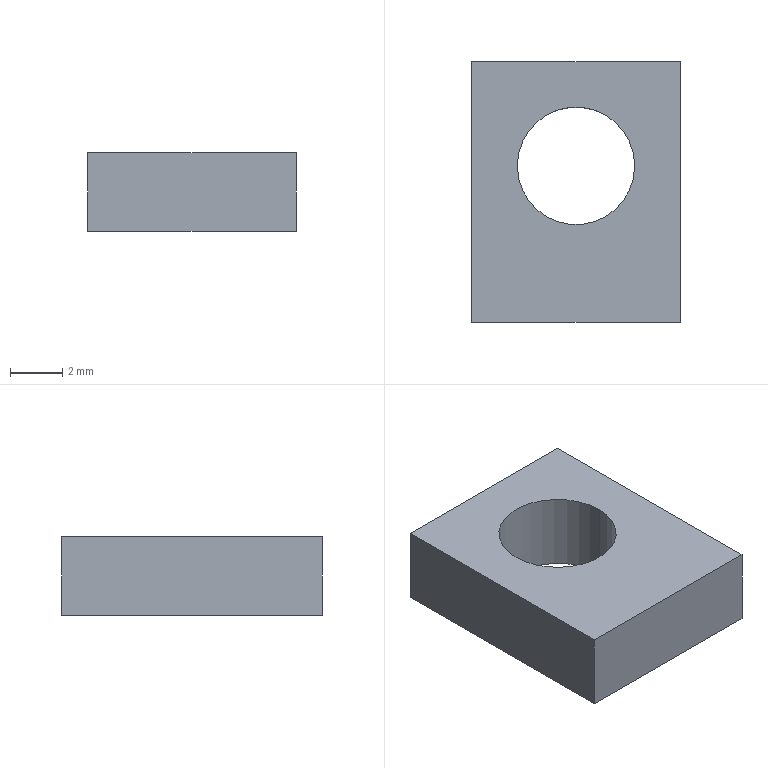Part | STEP file | Stopper plate | 1 solid | 8 faces | box 8 x 10 x 3 mm | volume 192.287 mm3 | plane 6 | cylinder 2 | commonest cylinder face diameters 4.5 x2
STEP:
#1=CARTESIAN_POINT('',(0.,0.,0.));
#2=DIRECTION('',(0.,0.,1.));
#3=DIRECTION('',(1.,0.,0.));
#4=AXIS2_PLACEMENT_3D('',#1,#2,#3);
#5=CARTESIAN_POINT('',(6.25,3.574,0.));
#6=VERTEX_POINT('',#5);
#7=CARTESIAN_POINT('',(6.25,3.574,3.));
#8=VERTEX_POINT('',#7);
#9=CARTESIAN_POINT('',(6.25,3.574,0.));
#10=DIRECTION('',(0.,0.,1.));
#11=VECTOR('',#10,1.);
#12=LINE('',#9,#11);
#13=CARTESIAN_POINT('',(4.,3.574,0.));
#14=DIRECTION('',(0.,0.,1.));
#15=DIRECTION('',(1.,0.,0.));
#16=AXIS2_PLACEMENT_3D('',#13,#14,#15);
#17=CYLINDRICAL_SURFACE('',#16,2.25);
#18=CARTESIAN_POINT('',(6.283,0.));
#19=DIRECTION('',(0.,1.));
#20=VECTOR('',#19,1.);
#21=LINE('',#18,#20);
#22=(GEOMETRIC_REPRESENTATION_CONTEXT(2)PARAMETRIC_REPRESENTATION_CONTEXT()REPRESENTATION_CONTEXT('',''));
#23=DEFINITIONAL_REPRESENTATION('',(#21),#22);
#24=PCURVE('',#17,#23);
#25=CARTESIAN_POINT('',(4.,3.574,0.));
#26=DIRECTION('',(0.,0.,1.));
#27=DIRECTION('',(1.,0.,0.));
#28=AXIS2_PLACEMENT_3D('',#25,#26,#27);
#29=CYLINDRICAL_SURFACE('',#28,2.25);
#30=CARTESIAN_POINT('',(0.,0.));
#31=DIRECTION('',(0.,1.));
#32=VECTOR('',#31,1.);
#33=LINE('',#30,#32);
#34=(GEOMETRIC_REPRESENTATION_CONTEXT(2)PARAMETRIC_REPRESENTATION_CONTEXT()REPRESENTATION_CONTEXT('',''));
#35=DEFINITIONAL_REPRESENTATION('',(#33),#34);
#36=PCURVE('',#29,#35);
#37=SURFACE_CURVE('',#12,(#24,#36),.PCURVE_S1.);
#38=EDGE_CURVE('',#6,#8,#37,.T.);
#39=ORIENTED_EDGE('',*,*,#38,.T.);
#40=CARTESIAN_POINT('',(1.75,3.574,3.));
#41=VERTEX_POINT('',#40);
#42=CARTESIAN_POINT('',(4.,3.574,3.));
#43=DIRECTION('',(0.,0.,1.));
#44=DIRECTION('',(1.,0.,0.));
#45=AXIS2_PLACEMENT_3D('',#42,#43,#44);
#46=CIRCLE('',#45,2.25);
#47=CARTESIAN_POINT('',(0.,3.));
#48=DIRECTION('',(1.,0.));
#49=VECTOR('',#48,1.);
#50=LINE('',#47,#49);
#51=(GEOMETRIC_REPRESENTATION_CONTEXT(2)PARAMETRIC_REPRESENTATION_CONTEXT()REPRESENTATION_CONTEXT('',''));
#52=DEFINITIONAL_REPRESENTATION('',(#50),#51);
#53=PCURVE('',#17,#52);
#54=CARTESIAN_POINT('',(0.,7.574,3.));
#55=DIRECTION('',(0.,0.,-1.));
#56=DIRECTION('',(-1.,0.,0.));
#57=AXIS2_PLACEMENT_3D('',#54,#55,#56);
#58=PLANE('',#57);
#59=CARTESIAN_POINT('',(-6.25,-4.));
#60=CARTESIAN_POINT('',(-6.25,-0.1029));
#61=CARTESIAN_POINT('',(-2.875,-2.051));
#62=CARTESIAN_POINT('',(0.5,-4.));
#63=CARTESIAN_POINT('',(-2.875,-5.949));
#64=CARTESIAN_POINT('',(-6.25,-7.897));
#65=CARTESIAN_POINT('',(-6.25,-4.));
#66=(BOUNDED_CURVE()B_SPLINE_CURVE(2,(#59,#60,#61,#62,#63,#64,#65),.UNSPECIFIED.,.T.,.F.)B_SPLINE_CURVE_WITH_KNOTS((1,2,2,2,2,1),(-2.094,0.,2.094,4.189,6.283,8.378),.UNSPECIFIED.)CURVE()GEOMETRIC_REPRESENTATION_ITEM()RATIONAL_B_SPLINE_CURVE((1.,0.5,1.,0.5,1.,0.5,1.))REPRESENTATION_ITEM(''));
#67=(GEOMETRIC_REPRESENTATION_CONTEXT(2)PARAMETRIC_REPRESENTATION_CONTEXT()REPRESENTATION_CONTEXT('',''));
#68=DEFINITIONAL_REPRESENTATION('',(#66),#67);
#69=PCURVE('',#58,#68);
#70=SURFACE_CURVE('',#46,(#53,#69),.PCURVE_S1.);
#71=EDGE_CURVE('',#41,#8,#70,.T.);
#72=ORIENTED_EDGE('',*,*,#71,.F.);
#73=CARTESIAN_POINT('',(1.75,3.574,0.));
#74=VERTEX_POINT('',#73);
#75=CARTESIAN_POINT('',(1.75,3.574,0.));
#76=DIRECTION('',(0.,0.,1.));
#77=VECTOR('',#76,1.);
#78=LINE('',#75,#77);
#79=CARTESIAN_POINT('',(3.142,0.));
#80=DIRECTION('',(0.,1.));
#81=VECTOR('',#80,1.);
#82=LINE('',#79,#81);
#83=(GEOMETRIC_REPRESENTATION_CONTEXT(2)PARAMETRIC_REPRESENTATION_CONTEXT()REPRESENTATION_CONTEXT('',''));
#84=DEFINITIONAL_REPRESENTATION('',(#82),#83);
#85=PCURVE('',#17,#84);
#86=CARTESIAN_POINT('',(3.142,0.));
#87=DIRECTION('',(0.,1.));
#88=VECTOR('',#87,1.);
#89=LINE('',#86,#88);
#90=(GEOMETRIC_REPRESENTATION_CONTEXT(2)PARAMETRIC_REPRESENTATION_CONTEXT()REPRESENTATION_CONTEXT('',''));
#91=DEFINITIONAL_REPRESENTATION('',(#89),#90);
#92=PCURVE('',#29,#91);
#93=SURFACE_CURVE('',#78,(#85,#92),.PCURVE_S1.);
#94=EDGE_CURVE('',#74,#41,#93,.T.);
#95=ORIENTED_EDGE('',*,*,#94,.F.);
#96=CARTESIAN_POINT('',(4.,3.574,0.));
#97=DIRECTION('',(0.,0.,1.));
#98=DIRECTION('',(1.,0.,0.));
#99=AXIS2_PLACEMENT_3D('',#96,#97,#98);
#100=CIRCLE('',#99,2.25);
#101=CARTESIAN_POINT('',(0.,0.));
#102=DIRECTION('',(1.,0.));
#103=VECTOR('',#102,1.);
#104=LINE('',#101,#103);
#105=(GEOMETRIC_REPRESENTATION_CONTEXT(2)PARAMETRIC_REPRESENTATION_CONTEXT()REPRESENTATION_CONTEXT('',''));
#106=DEFINITIONAL_REPRESENTATION('',(#104),#105);
#107=PCURVE('',#17,#106);
#108=CARTESIAN_POINT('',(0.,7.574,0.));
#109=DIRECTION('',(0.,0.,-1.));
#110=DIRECTION('',(-1.,0.,0.));
#111=AXIS2_PLACEMENT_3D('',#108,#109,#110);
#112=PLANE('',#111);
#113=CARTESIAN_POINT('',(-6.25,-4.));
#114=CARTESIAN_POINT('',(-6.25,-0.1029));
#115=CARTESIAN_POINT('',(-2.875,-2.051));
#116=CARTESIAN_POINT('',(0.5,-4.));
#117=CARTESIAN_POINT('',(-2.875,-5.949));
#118=CARTESIAN_POINT('',(-6.25,-7.897));
#119=CARTESIAN_POINT('',(-6.25,-4.));
#120=(BOUNDED_CURVE()B_SPLINE_CURVE(2,(#113,#114,#115,#116,#117,#118,#119),.UNSPECIFIED.,.T.,.F.)B_SPLINE_CURVE_WITH_KNOTS((1,2,2,2,2,1),(-2.094,0.,2.094,4.189,6.283,8.378),.UNSPECIFIED.)CURVE()GEOMETRIC_REPRESENTATION_ITEM()RATIONAL_B_SPLINE_CURVE((1.,0.5,1.,0.5,1.,0.5,1.))REPRESENTATION_ITEM(''));
#121=(GEOMETRIC_REPRESENTATION_CONTEXT(2)PARAMETRIC_REPRESENTATION_CONTEXT()REPRESENTATION_CONTEXT('',''));
#122=DEFINITIONAL_REPRESENTATION('',(#120),#121);
#123=PCURVE('',#112,#122);
#124=SURFACE_CURVE('',#100,(#107,#123),.PCURVE_S1.);
#125=EDGE_CURVE('',#74,#6,#124,.T.);
#126=ORIENTED_EDGE('',*,*,#125,.T.);
#127=EDGE_LOOP('',(#39,#72,#95,#126));
#128=FACE_BOUND('',#127,.F.);
#129=ADVANCED_FACE('',(#128),#17,.F.);
#130=CARTESIAN_POINT('',(0.,7.574,0.));
#131=VERTEX_POINT('',#130);
#132=CARTESIAN_POINT('',(0.,-2.426,0.));
#133=VERTEX_POINT('',#132);
#134=CARTESIAN_POINT('',(0.,-2.426,0.));
#135=DIRECTION('',(0.,-1.,0.));
#136=VECTOR('',#135,1.);
#137=LINE('',#134,#136);
#138=CARTESIAN_POINT('',(0.,-2.426,3.));
#139=DIRECTION('',(1.,0.,0.));
#140=DIRECTION('',(0.,0.,-1.));
#141=AXIS2_PLACEMENT_3D('',#138,#139,#140);
#142=PLANE('',#141);
#143=CARTESIAN_POINT('',(3.,0.));
#144=DIRECTION('',(0.,-1.));
#145=VECTOR('',#144,1.);
#146=LINE('',#143,#145);
#147=(GEOMETRIC_REPRESENTATION_CONTEXT(2)PARAMETRIC_REPRESENTATION_CONTEXT()REPRESENTATION_CONTEXT('',''));
#148=DEFINITIONAL_REPRESENTATION('',(#146),#147);
#149=PCURVE('',#142,#148);
#150=CARTESIAN_POINT('',(0.,-10.));
#151=DIRECTION('',(0.,-1.));
#152=VECTOR('',#151,1.);
#153=LINE('',#150,#152);
#154=(GEOMETRIC_REPRESENTATION_CONTEXT(2)PARAMETRIC_REPRESENTATION_CONTEXT()REPRESENTATION_CONTEXT('',''));
#155=DEFINITIONAL_REPRESENTATION('',(#153),#154);
#156=PCURVE('',#112,#155);
#157=SURFACE_CURVE('',#137,(#149,#156),.PCURVE_S1.);
#158=EDGE_CURVE('',#131,#133,#157,.T.);
#159=ORIENTED_EDGE('',*,*,#158,.T.);
#160=CARTESIAN_POINT('',(0.,-2.426,3.));
#161=VERTEX_POINT('',#160);
#162=CARTESIAN_POINT('',(0.,-2.426,3.));
#163=DIRECTION('',(0.,0.,-1.));
#164=VECTOR('',#163,1.);
#165=LINE('',#162,#164);
#166=CARTESIAN_POINT('',(0.,0.));
#167=DIRECTION('',(1.,0.));
#168=VECTOR('',#167,1.);
#169=LINE('',#166,#168);
#170=(GEOMETRIC_REPRESENTATION_CONTEXT(2)PARAMETRIC_REPRESENTATION_CONTEXT()REPRESENTATION_CONTEXT('',''));
#171=DEFINITIONAL_REPRESENTATION('',(#169),#170);
#172=PCURVE('',#142,#171);
#173=CARTESIAN_POINT('',(0.,-2.426,3.));
#174=DIRECTION('',(0.,1.,0.));
#175=DIRECTION('',(0.,0.,1.));
#176=AXIS2_PLACEMENT_3D('',#173,#174,#175);
#177=PLANE('',#176);
#178=CARTESIAN_POINT('',(0.,0.));
#179=DIRECTION('',(-1.,0.));
#180=VECTOR('',#179,1.);
#181=LINE('',#178,#180);
#182=(GEOMETRIC_REPRESENTATION_CONTEXT(2)PARAMETRIC_REPRESENTATION_CONTEXT()REPRESENTATION_CONTEXT('',''));
#183=DEFINITIONAL_REPRESENTATION('',(#181),#182);
#184=PCURVE('',#177,#183);
#185=SURFACE_CURVE('',#165,(#172,#184),.PCURVE_S1.);
#186=EDGE_CURVE('',#161,#133,#185,.T.);
#187=ORIENTED_EDGE('',*,*,#186,.F.);
#188=CARTESIAN_POINT('',(0.,7.574,3.));
#189=VERTEX_POINT('',#188);
#190=CARTESIAN_POINT('',(0.,-2.426,3.));
#191=DIRECTION('',(0.,-1.,0.));
#192=VECTOR('',#191,1.);
#193=LINE('',#190,#192);
#194=CARTESIAN_POINT('',(0.,0.));
#195=DIRECTION('',(0.,-1.));
#196=VECTOR('',#195,1.);
#197=LINE('',#194,#196);
#198=(GEOMETRIC_REPRESENTATION_CONTEXT(2)PARAMETRIC_REPRESENTATION_CONTEXT()REPRESENTATION_CONTEXT('',''));
#199=DEFINITIONAL_REPRESENTATION('',(#197),#198);
#200=PCURVE('',#142,#199);
#201=CARTESIAN_POINT('',(0.,-10.));
#202=DIRECTION('',(0.,-1.));
#203=VECTOR('',#202,1.);
#204=LINE('',#201,#203);
#205=(GEOMETRIC_REPRESENTATION_CONTEXT(2)PARAMETRIC_REPRESENTATION_CONTEXT()REPRESENTATION_CONTEXT('',''));
#206=DEFINITIONAL_REPRESENTATION('',(#204),#205);
#207=PCURVE('',#58,#206);
#208=SURFACE_CURVE('',#193,(#200,#207),.PCURVE_S1.);
#209=EDGE_CURVE('',#189,#161,#208,.T.);
#210=ORIENTED_EDGE('',*,*,#209,.F.);
#211=CARTESIAN_POINT('',(0.,7.574,3.));
#212=DIRECTION('',(0.,0.,-1.));
#213=VECTOR('',#212,1.);
#214=LINE('',#211,#213);
#215=CARTESIAN_POINT('',(0.,10.));
#216=DIRECTION('',(1.,0.));
#217=VECTOR('',#216,1.);
#218=LINE('',#215,#217);
#219=(GEOMETRIC_REPRESENTATION_CONTEXT(2)PARAMETRIC_REPRESENTATION_CONTEXT()REPRESENTATION_CONTEXT('',''));
#220=DEFINITIONAL_REPRESENTATION('',(#218),#219);
#221=PCURVE('',#142,#220);
#222=CARTESIAN_POINT('',(0.,7.574,3.));
#223=DIRECTION('',(0.,-1.,0.));
#224=DIRECTION('',(0.,0.,-1.));
#225=AXIS2_PLACEMENT_3D('',#222,#223,#224);
#226=PLANE('',#225);
#227=CARTESIAN_POINT('',(0.,0.));
#228=DIRECTION('',(1.,0.));
#229=VECTOR('',#228,1.);
#230=LINE('',#227,#229);
#231=(GEOMETRIC_REPRESENTATION_CONTEXT(2)PARAMETRIC_REPRESENTATION_CONTEXT()REPRESENTATION_CONTEXT('',''));
#232=DEFINITIONAL_REPRESENTATION('',(#230),#231);
#233=PCURVE('',#226,#232);
#234=SURFACE_CURVE('',#214,(#221,#233),.PCURVE_S1.);
#235=EDGE_CURVE('',#189,#131,#234,.T.);
#236=ORIENTED_EDGE('',*,*,#235,.T.);
#237=EDGE_LOOP('',(#159,#187,#210,#236));
#238=FACE_BOUND('',#237,.T.);
#239=ADVANCED_FACE('',(#238),#142,.F.);
#240=CARTESIAN_POINT('',(8.,-2.426,0.));
#241=VERTEX_POINT('',#240);
#242=CARTESIAN_POINT('',(0.,-2.426,0.));
#243=DIRECTION('',(1.,0.,0.));
#244=VECTOR('',#243,1.);
#245=LINE('',#242,#244);
#246=CARTESIAN_POINT('',(-3.,0.));
#247=DIRECTION('',(0.,1.));
#248=VECTOR('',#247,1.);
#249=LINE('',#246,#248);
#250=(GEOMETRIC_REPRESENTATION_CONTEXT(2)PARAMETRIC_REPRESENTATION_CONTEXT()REPRESENTATION_CONTEXT('',''));
#251=DEFINITIONAL_REPRESENTATION('',(#249),#250);
#252=PCURVE('',#177,#251);
#253=CARTESIAN_POINT('',(0.,-10.));
#254=DIRECTION('',(-1.,0.));
#255=VECTOR('',#254,1.);
#256=LINE('',#253,#255);
#257=(GEOMETRIC_REPRESENTATION_CONTEXT(2)PARAMETRIC_REPRESENTATION_CONTEXT()REPRESENTATION_CONTEXT('',''));
#258=DEFINITIONAL_REPRESENTATION('',(#256),#257);
#259=PCURVE('',#112,#258);
#260=SURFACE_CURVE('',#245,(#252,#259),.PCURVE_S1.);
#261=EDGE_CURVE('',#133,#241,#260,.T.);
#262=ORIENTED_EDGE('',*,*,#261,.T.);
#263=CARTESIAN_POINT('',(8.,-2.426,3.));
#264=VERTEX_POINT('',#263);
#265=CARTESIAN_POINT('',(8.,-2.426,3.));
#266=DIRECTION('',(0.,0.,-1.));
#267=VECTOR('',#266,1.);
#268=LINE('',#265,#267);
#269=CARTESIAN_POINT('',(0.,8.));
#270=DIRECTION('',(-1.,0.));
#271=VECTOR('',#270,1.);
#272=LINE('',#269,#271);
#273=(GEOMETRIC_REPRESENTATION_CONTEXT(2)PARAMETRIC_REPRESENTATION_CONTEXT()REPRESENTATION_CONTEXT('',''));
#274=DEFINITIONAL_REPRESENTATION('',(#272),#273);
#275=PCURVE('',#177,#274);
#276=CARTESIAN_POINT('',(8.,-2.426,3.));
#277=DIRECTION('',(-1.,0.,0.));
#278=DIRECTION('',(0.,0.,1.));
#279=AXIS2_PLACEMENT_3D('',#276,#277,#278);
#280=PLANE('',#279);
#281=CARTESIAN_POINT('',(0.,0.));
#282=DIRECTION('',(-1.,0.));
#283=VECTOR('',#282,1.);
#284=LINE('',#281,#283);
#285=(GEOMETRIC_REPRESENTATION_CONTEXT(2)PARAMETRIC_REPRESENTATION_CONTEXT()REPRESENTATION_CONTEXT('',''));
#286=DEFINITIONAL_REPRESENTATION('',(#284),#285);
#287=PCURVE('',#280,#286);
#288=SURFACE_CURVE('',#268,(#275,#287),.PCURVE_S1.);
#289=EDGE_CURVE('',#264,#241,#288,.T.);
#290=ORIENTED_EDGE('',*,*,#289,.F.);
#291=CARTESIAN_POINT('',(0.,-2.426,3.));
#292=DIRECTION('',(1.,0.,0.));
#293=VECTOR('',#292,1.);
#294=LINE('',#291,#293);
#295=CARTESIAN_POINT('',(0.,0.));
#296=DIRECTION('',(0.,1.));
#297=VECTOR('',#296,1.);
#298=LINE('',#295,#297);
#299=(GEOMETRIC_REPRESENTATION_CONTEXT(2)PARAMETRIC_REPRESENTATION_CONTEXT()REPRESENTATION_CONTEXT('',''));
#300=DEFINITIONAL_REPRESENTATION('',(#298),#299);
#301=PCURVE('',#177,#300);
#302=CARTESIAN_POINT('',(0.,-10.));
#303=DIRECTION('',(-1.,0.));
#304=VECTOR('',#303,1.);
#305=LINE('',#302,#304);
#306=(GEOMETRIC_REPRESENTATION_CONTEXT(2)PARAMETRIC_REPRESENTATION_CONTEXT()REPRESENTATION_CONTEXT('',''));
#307=DEFINITIONAL_REPRESENTATION('',(#305),#306);
#308=PCURVE('',#58,#307);
#309=SURFACE_CURVE('',#294,(#301,#308),.PCURVE_S1.);
#310=EDGE_CURVE('',#161,#264,#309,.T.);
#311=ORIENTED_EDGE('',*,*,#310,.F.);
#312=ORIENTED_EDGE('',*,*,#186,.T.);
#313=EDGE_LOOP('',(#262,#290,#311,#312));
#314=FACE_BOUND('',#313,.T.);
#315=ADVANCED_FACE('',(#314),#177,.F.);
#316=CARTESIAN_POINT('',(8.,7.574,0.));
#317=VERTEX_POINT('',#316);
#318=CARTESIAN_POINT('',(8.,-2.426,0.));
#319=DIRECTION('',(0.,1.,0.));
#320=VECTOR('',#319,1.);
#321=LINE('',#318,#320);
#322=CARTESIAN_POINT('',(-3.,0.));
#323=DIRECTION('',(0.,1.));
#324=VECTOR('',#323,1.);
#325=LINE('',#322,#324);
#326=(GEOMETRIC_REPRESENTATION_CONTEXT(2)PARAMETRIC_REPRESENTATION_CONTEXT()REPRESENTATION_CONTEXT('',''));
#327=DEFINITIONAL_REPRESENTATION('',(#325),#326);
#328=PCURVE('',#280,#327);
#329=CARTESIAN_POINT('',(-8.,-10.));
#330=DIRECTION('',(0.,1.));
#331=VECTOR('',#330,1.);
#332=LINE('',#329,#331);
#333=(GEOMETRIC_REPRESENTATION_CONTEXT(2)PARAMETRIC_REPRESENTATION_CONTEXT()REPRESENTATION_CONTEXT('',''));
#334=DEFINITIONAL_REPRESENTATION('',(#332),#333);
#335=PCURVE('',#112,#334);
#336=SURFACE_CURVE('',#321,(#328,#335),.PCURVE_S1.);
#337=EDGE_CURVE('',#241,#317,#336,.T.);
#338=ORIENTED_EDGE('',*,*,#337,.T.);
#339=CARTESIAN_POINT('',(8.,7.574,3.));
#340=VERTEX_POINT('',#339);
#341=CARTESIAN_POINT('',(8.,7.574,3.));
#342=DIRECTION('',(0.,0.,-1.));
#343=VECTOR('',#342,1.);
#344=LINE('',#341,#343);
#345=CARTESIAN_POINT('',(0.,10.));
#346=DIRECTION('',(-1.,0.));
#347=VECTOR('',#346,1.);
#348=LINE('',#345,#347);
#349=(GEOMETRIC_REPRESENTATION_CONTEXT(2)PARAMETRIC_REPRESENTATION_CONTEXT()REPRESENTATION_CONTEXT('',''));
#350=DEFINITIONAL_REPRESENTATION('',(#348),#349);
#351=PCURVE('',#280,#350);
#352=CARTESIAN_POINT('',(0.,8.));
#353=DIRECTION('',(1.,0.));
#354=VECTOR('',#353,1.);
#355=LINE('',#352,#354);
#356=(GEOMETRIC_REPRESENTATION_CONTEXT(2)PARAMETRIC_REPRESENTATION_CONTEXT()REPRESENTATION_CONTEXT('',''));
#357=DEFINITIONAL_REPRESENTATION('',(#355),#356);
#358=PCURVE('',#226,#357);
#359=SURFACE_CURVE('',#344,(#351,#358),.PCURVE_S1.);
#360=EDGE_CURVE('',#340,#317,#359,.T.);
#361=ORIENTED_EDGE('',*,*,#360,.F.);
#362=CARTESIAN_POINT('',(8.,-2.426,3.));
#363=DIRECTION('',(0.,1.,0.));
#364=VECTOR('',#363,1.);
#365=LINE('',#362,#364);
#366=CARTESIAN_POINT('',(0.,0.));
#367=DIRECTION('',(0.,1.));
#368=VECTOR('',#367,1.);
#369=LINE('',#366,#368);
#370=(GEOMETRIC_REPRESENTATION_CONTEXT(2)PARAMETRIC_REPRESENTATION_CONTEXT()REPRESENTATION_CONTEXT('',''));
#371=DEFINITIONAL_REPRESENTATION('',(#369),#370);
#372=PCURVE('',#280,#371);
#373=CARTESIAN_POINT('',(-8.,-10.));
#374=DIRECTION('',(0.,1.));
#375=VECTOR('',#374,1.);
#376=LINE('',#373,#375);
#377=(GEOMETRIC_REPRESENTATION_CONTEXT(2)PARAMETRIC_REPRESENTATION_CONTEXT()REPRESENTATION_CONTEXT('',''));
#378=DEFINITIONAL_REPRESENTATION('',(#376),#377);
#379=PCURVE('',#58,#378);
#380=SURFACE_CURVE('',#365,(#372,#379),.PCURVE_S1.);
#381=EDGE_CURVE('',#264,#340,#380,.T.);
#382=ORIENTED_EDGE('',*,*,#381,.F.);
#383=ORIENTED_EDGE('',*,*,#289,.T.);
#384=EDGE_LOOP('',(#338,#361,#382,#383));
#385=FACE_BOUND('',#384,.T.);
#386=ADVANCED_FACE('',(#385),#280,.F.);
#387=CARTESIAN_POINT('',(0.,7.574,0.));
#388=DIRECTION('',(-1.,0.,0.));
#389=VECTOR('',#388,1.);
#390=LINE('',#387,#389);
#391=CARTESIAN_POINT('',(3.,0.));
#392=DIRECTION('',(0.,-1.));
#393=VECTOR('',#392,1.);
#394=LINE('',#391,#393);
#395=(GEOMETRIC_REPRESENTATION_CONTEXT(2)PARAMETRIC_REPRESENTATION_CONTEXT()REPRESENTATION_CONTEXT('',''));
#396=DEFINITIONAL_REPRESENTATION('',(#394),#395);
#397=PCURVE('',#226,#396);
#398=CARTESIAN_POINT('',(0.,0.));
#399=DIRECTION('',(1.,0.));
#400=VECTOR('',#399,1.);
#401=LINE('',#398,#400);
#402=(GEOMETRIC_REPRESENTATION_CONTEXT(2)PARAMETRIC_REPRESENTATION_CONTEXT()REPRESENTATION_CONTEXT('',''));
#403=DEFINITIONAL_REPRESENTATION('',(#401),#402);
#404=PCURVE('',#112,#403);
#405=SURFACE_CURVE('',#390,(#397,#404),.PCURVE_S1.);
#406=EDGE_CURVE('',#317,#131,#405,.T.);
#407=ORIENTED_EDGE('',*,*,#406,.T.);
#408=ORIENTED_EDGE('',*,*,#235,.F.);
#409=CARTESIAN_POINT('',(0.,7.574,3.));
#410=DIRECTION('',(-1.,0.,0.));
#411=VECTOR('',#410,1.);
#412=LINE('',#409,#411);
#413=CARTESIAN_POINT('',(0.,0.));
#414=DIRECTION('',(0.,-1.));
#415=VECTOR('',#414,1.);
#416=LINE('',#413,#415);
#417=(GEOMETRIC_REPRESENTATION_CONTEXT(2)PARAMETRIC_REPRESENTATION_CONTEXT()REPRESENTATION_CONTEXT('',''));
#418=DEFINITIONAL_REPRESENTATION('',(#416),#417);
#419=PCURVE('',#226,#418);
#420=CARTESIAN_POINT('',(0.,0.));
#421=DIRECTION('',(1.,0.));
#422=VECTOR('',#421,1.);
#423=LINE('',#420,#422);
#424=(GEOMETRIC_REPRESENTATION_CONTEXT(2)PARAMETRIC_REPRESENTATION_CONTEXT()REPRESENTATION_CONTEXT('',''));
#425=DEFINITIONAL_REPRESENTATION('',(#423),#424);
#426=PCURVE('',#58,#425);
#427=SURFACE_CURVE('',#412,(#419,#426),.PCURVE_S1.);
#428=EDGE_CURVE('',#340,#189,#427,.T.);
#429=ORIENTED_EDGE('',*,*,#428,.F.);
#430=ORIENTED_EDGE('',*,*,#360,.T.);
#431=EDGE_LOOP('',(#407,#408,#429,#430));
#432=FACE_BOUND('',#431,.T.);
#433=ADVANCED_FACE('',(#432),#226,.F.);
#434=CARTESIAN_POINT('',(4.,3.574,3.));
#435=DIRECTION('',(0.,0.,1.));
#436=DIRECTION('',(1.,0.,0.));
#437=AXIS2_PLACEMENT_3D('',#434,#435,#436);
#438=CIRCLE('',#437,2.25);
#439=CARTESIAN_POINT('',(-6.25,-4.));
#440=CARTESIAN_POINT('',(-6.25,-0.1029));
#441=CARTESIAN_POINT('',(-2.875,-2.051));
#442=CARTESIAN_POINT('',(0.5,-4.));
#443=CARTESIAN_POINT('',(-2.875,-5.949));
#444=CARTESIAN_POINT('',(-6.25,-7.897));
#445=CARTESIAN_POINT('',(-6.25,-4.));
#446=(BOUNDED_CURVE()B_SPLINE_CURVE(2,(#439,#440,#441,#442,#443,#444,#445),.UNSPECIFIED.,.T.,.F.)B_SPLINE_CURVE_WITH_KNOTS((1,2,2,2,2,1),(-2.094,0.,2.094,4.189,6.283,8.378),.UNSPECIFIED.)CURVE()GEOMETRIC_REPRESENTATION_ITEM()RATIONAL_B_SPLINE_CURVE((1.,0.5,1.,0.5,1.,0.5,1.))REPRESENTATION_ITEM(''));
#447=(GEOMETRIC_REPRESENTATION_CONTEXT(2)PARAMETRIC_REPRESENTATION_CONTEXT()REPRESENTATION_CONTEXT('',''));
#448=DEFINITIONAL_REPRESENTATION('',(#446),#447);
#449=PCURVE('',#58,#448);
#450=CARTESIAN_POINT('',(0.,3.));
#451=DIRECTION('',(1.,0.));
#452=VECTOR('',#451,1.);
#453=LINE('',#450,#452);
#454=(GEOMETRIC_REPRESENTATION_CONTEXT(2)PARAMETRIC_REPRESENTATION_CONTEXT()REPRESENTATION_CONTEXT('',''));
#455=DEFINITIONAL_REPRESENTATION('',(#453),#454);
#456=PCURVE('',#29,#455);
#457=SURFACE_CURVE('',#438,(#449,#456),.PCURVE_S1.);
#458=EDGE_CURVE('',#8,#41,#457,.T.);
#459=ORIENTED_EDGE('',*,*,#458,.F.);
#460=ORIENTED_EDGE('',*,*,#71,.F.);
#461=EDGE_LOOP('',(#459,#460));
#462=FACE_BOUND('',#461,.T.);
#463=ORIENTED_EDGE('',*,*,#209,.T.);
#464=ORIENTED_EDGE('',*,*,#310,.T.);
#465=ORIENTED_EDGE('',*,*,#381,.T.);
#466=ORIENTED_EDGE('',*,*,#428,.T.);
#467=EDGE_LOOP('',(#463,#464,#465,#466));
#468=FACE_BOUND('',#467,.T.);
#469=ADVANCED_FACE('',(#462,#468),#58,.F.);
#470=CARTESIAN_POINT('',(4.,3.574,0.));
#471=DIRECTION('',(0.,0.,1.));
#472=DIRECTION('',(1.,0.,0.));
#473=AXIS2_PLACEMENT_3D('',#470,#471,#472);
#474=CIRCLE('',#473,2.25);
#475=CARTESIAN_POINT('',(-6.25,-4.));
#476=CARTESIAN_POINT('',(-6.25,-0.1029));
#477=CARTESIAN_POINT('',(-2.875,-2.051));
#478=CARTESIAN_POINT('',(0.5,-4.));
#479=CARTESIAN_POINT('',(-2.875,-5.949));
#480=CARTESIAN_POINT('',(-6.25,-7.897));
#481=CARTESIAN_POINT('',(-6.25,-4.));
#482=(BOUNDED_CURVE()B_SPLINE_CURVE(2,(#475,#476,#477,#478,#479,#480,#481),.UNSPECIFIED.,.T.,.F.)B_SPLINE_CURVE_WITH_KNOTS((1,2,2,2,2,1),(-2.094,0.,2.094,4.189,6.283,8.378),.UNSPECIFIED.)CURVE()GEOMETRIC_REPRESENTATION_ITEM()RATIONAL_B_SPLINE_CURVE((1.,0.5,1.,0.5,1.,0.5,1.))REPRESENTATION_ITEM(''));
#483=(GEOMETRIC_REPRESENTATION_CONTEXT(2)PARAMETRIC_REPRESENTATION_CONTEXT()REPRESENTATION_CONTEXT('',''));
#484=DEFINITIONAL_REPRESENTATION('',(#482),#483);
#485=PCURVE('',#112,#484);
#486=CARTESIAN_POINT('',(0.,0.));
#487=DIRECTION('',(1.,0.));
#488=VECTOR('',#487,1.);
#489=LINE('',#486,#488);
#490=(GEOMETRIC_REPRESENTATION_CONTEXT(2)PARAMETRIC_REPRESENTATION_CONTEXT()REPRESENTATION_CONTEXT('',''));
#491=DEFINITIONAL_REPRESENTATION('',(#489),#490);
#492=PCURVE('',#29,#491);
#493=SURFACE_CURVE('',#474,(#485,#492),.PCURVE_S1.);
#494=EDGE_CURVE('',#6,#74,#493,.T.);
#495=ORIENTED_EDGE('',*,*,#494,.T.);
#496=ORIENTED_EDGE('',*,*,#125,.T.);
#497=EDGE_LOOP('',(#495,#496));
#498=FACE_BOUND('',#497,.T.);
#499=ORIENTED_EDGE('',*,*,#158,.F.);
#500=ORIENTED_EDGE('',*,*,#406,.F.);
#501=ORIENTED_EDGE('',*,*,#337,.F.);
#502=ORIENTED_EDGE('',*,*,#261,.F.);
#503=EDGE_LOOP('',(#499,#500,#501,#502));
#504=FACE_BOUND('',#503,.T.);
#505=ADVANCED_FACE('',(#498,#504),#112,.T.);
#506=ORIENTED_EDGE('',*,*,#458,.F.);
#507=ORIENTED_EDGE('',*,*,#38,.F.);
#508=ORIENTED_EDGE('',*,*,#494,.T.);
#509=ORIENTED_EDGE('',*,*,#94,.T.);
#510=EDGE_LOOP('',(#506,#507,#508,#509));
#511=FACE_BOUND('',#510,.F.);
#512=ADVANCED_FACE('',(#511),#29,.F.);
#513=CLOSED_SHELL('',(#129,#239,#315,#386,#433,#469,#505,#512));
#514=MANIFOLD_SOLID_BREP('',#513);
#515=(LENGTH_UNIT()NAMED_UNIT(*)SI_UNIT(.MILLI.,.METRE.));
#516=UNCERTAINTY_MEASURE_WITH_UNIT(LENGTH_MEASURE(0.0000001),#515,'','');
#517=(NAMED_UNIT(*)PLANE_ANGLE_UNIT()SI_UNIT($,.RADIAN.));
#518=(NAMED_UNIT(*)SI_UNIT($,.STERADIAN.)SOLID_ANGLE_UNIT());
#519=(GEOMETRIC_REPRESENTATION_CONTEXT(3)GLOBAL_UNCERTAINTY_ASSIGNED_CONTEXT((#516))GLOBAL_UNIT_ASSIGNED_CONTEXT((#515,#517,#518))REPRESENTATION_CONTEXT('',''));
#520=ADVANCED_BREP_SHAPE_REPRESENTATION('',(#4,#514),#519);